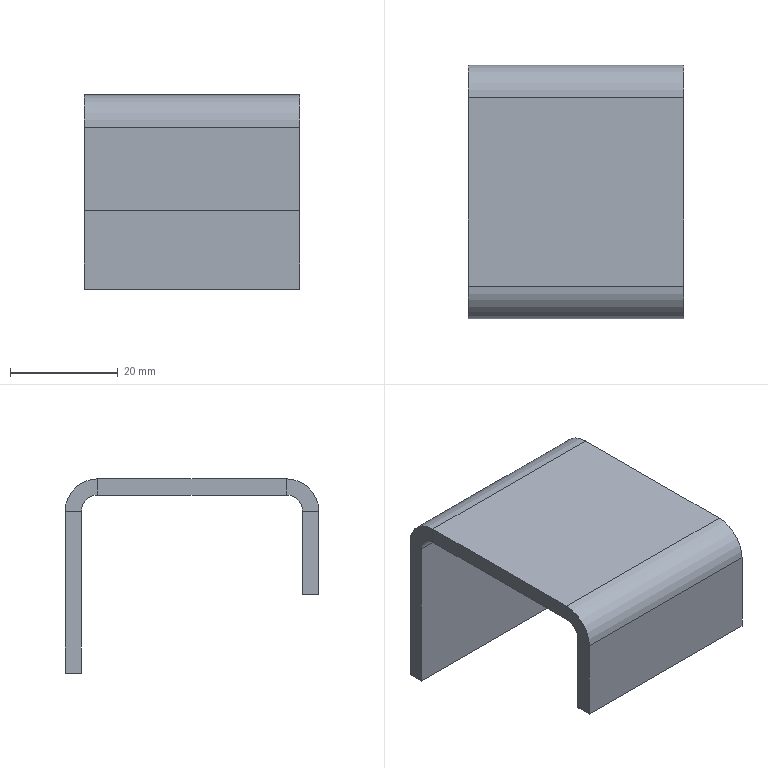Part | SolidWorks | features FlatPattern 1, SMBaseFlange 1, SheetMetal 1 | 1 solid | 22 faces | box 40 x 47 x 36 mm | volume 11356 mm3 | plane 18 | cylinder 4 | commonest cylinder face diameters 6 x2 12 x2
STEP:
#1=CARTESIAN_POINT('',(40.,0.,30.));
#2=VERTEX_POINT('',#1);
#3=CARTESIAN_POINT('',(40.,-3.,30.));
#4=VERTEX_POINT('',#3);
#5=CARTESIAN_POINT('',(40.,0.,30.));
#6=DIRECTION('',(0.,-1.,0.));
#7=VECTOR('',#6,1000.);
#8=LINE('',#5,#7);
#9=EDGE_CURVE('',#2,#4,#8,.T.);
#10=ORIENTED_EDGE('',*,*,#9,.F.);
#11=CARTESIAN_POINT('',(40.,-6.,36.));
#12=VERTEX_POINT('',#11);
#13=CARTESIAN_POINT('',(40.,-6.,30.));
#14=DIRECTION('',(1.,0.,0.));
#15=DIRECTION('',(0.,0.,1.));
#16=AXIS2_PLACEMENT_3D('',#13,#14,#15);
#17=CIRCLE('',#16,6.);
#18=EDGE_CURVE('',#2,#12,#17,.T.);
#19=ORIENTED_EDGE('',*,*,#18,.T.);
#20=CARTESIAN_POINT('',(40.,-6.,33.));
#21=VERTEX_POINT('',#20);
#22=CARTESIAN_POINT('',(40.,-6.,33.));
#23=DIRECTION('',(0.,0.,1.));
#24=VECTOR('',#23,1000.);
#25=LINE('',#22,#24);
#26=EDGE_CURVE('',#21,#12,#25,.T.);
#27=ORIENTED_EDGE('',*,*,#26,.F.);
#28=CARTESIAN_POINT('',(40.,-6.,30.));
#29=DIRECTION('',(1.,0.,0.));
#30=DIRECTION('',(0.,0.,-1.));
#31=AXIS2_PLACEMENT_3D('',#28,#29,#30);
#32=CIRCLE('',#31,3.);
#33=EDGE_CURVE('',#4,#21,#32,.T.);
#34=ORIENTED_EDGE('',*,*,#33,.F.);
#35=EDGE_LOOP('',(#10,#19,#27,#34));
#36=FACE_OUTER_BOUND('',#35,.T.);
#37=CARTESIAN_POINT('',(40.,0.,30.));
#38=DIRECTION('',(1.,0.,0.));
#39=DIRECTION('',(0.,0.,-1.));
#40=AXIS2_PLACEMENT_3D('',#37,#38,#39);
#41=PLANE('',#40);
#42=ADVANCED_FACE('',(#36),#41,.T.);
#43=CARTESIAN_POINT('',(40.,0.,0.));
#44=VERTEX_POINT('',#43);
#45=CARTESIAN_POINT('',(40.,0.,0.));
#46=DIRECTION('',(0.,0.,1.));
#47=VECTOR('',#46,1000.);
#48=LINE('',#45,#47);
#49=EDGE_CURVE('',#44,#2,#48,.T.);
#50=ORIENTED_EDGE('',*,*,#49,.T.);
#51=ORIENTED_EDGE('',*,*,#9,.T.);
#52=CARTESIAN_POINT('',(40.,-3.,0.));
#53=VERTEX_POINT('',#52);
#54=CARTESIAN_POINT('',(40.,-3.,0.));
#55=DIRECTION('',(0.,0.,1.));
#56=VECTOR('',#55,1000.);
#57=LINE('',#54,#56);
#58=EDGE_CURVE('',#53,#4,#57,.T.);
#59=ORIENTED_EDGE('',*,*,#58,.F.);
#60=CARTESIAN_POINT('',(40.,0.,0.));
#61=DIRECTION('',(0.,-1.,0.));
#62=VECTOR('',#61,1000.);
#63=LINE('',#60,#62);
#64=EDGE_CURVE('',#44,#53,#63,.T.);
#65=ORIENTED_EDGE('',*,*,#64,.F.);
#66=EDGE_LOOP('',(#50,#51,#59,#65));
#67=FACE_OUTER_BOUND('',#66,.T.);
#68=CARTESIAN_POINT('',(40.,-6.,33.));
#69=DIRECTION('',(1.,0.,0.));
#70=DIRECTION('',(0.,0.,-1.));
#71=AXIS2_PLACEMENT_3D('',#68,#69,#70);
#72=PLANE('',#71);
#73=ADVANCED_FACE('',(#67),#72,.T.);
#74=CARTESIAN_POINT('',(0.,-6.,36.));
#75=VERTEX_POINT('',#74);
#76=CARTESIAN_POINT('',(0.,-6.,33.));
#77=VERTEX_POINT('',#76);
#78=CARTESIAN_POINT('',(0.,-6.,36.));
#79=DIRECTION('',(0.,0.,-1.));
#80=VECTOR('',#79,1000.);
#81=LINE('',#78,#80);
#82=EDGE_CURVE('',#75,#77,#81,.T.);
#83=ORIENTED_EDGE('',*,*,#82,.F.);
#84=CARTESIAN_POINT('',(0.,0.,30.));
#85=VERTEX_POINT('',#84);
#86=CARTESIAN_POINT('',(0.,-6.,30.));
#87=DIRECTION('',(1.,0.,0.));
#88=DIRECTION('',(0.,0.,1.));
#89=AXIS2_PLACEMENT_3D('',#86,#87,#88);
#90=CIRCLE('',#89,6.);
#91=EDGE_CURVE('',#85,#75,#90,.T.);
#92=ORIENTED_EDGE('',*,*,#91,.F.);
#93=CARTESIAN_POINT('',(0.,-3.,30.));
#94=VERTEX_POINT('',#93);
#95=CARTESIAN_POINT('',(0.,-3.,30.));
#96=DIRECTION('',(0.,1.,0.));
#97=VECTOR('',#96,1000.);
#98=LINE('',#95,#97);
#99=EDGE_CURVE('',#94,#85,#98,.T.);
#100=ORIENTED_EDGE('',*,*,#99,.F.);
#101=CARTESIAN_POINT('',(0.,-6.,30.));
#102=DIRECTION('',(1.,0.,0.));
#103=DIRECTION('',(0.,0.,-1.));
#104=AXIS2_PLACEMENT_3D('',#101,#102,#103);
#105=CIRCLE('',#104,3.);
#106=EDGE_CURVE('',#94,#77,#105,.T.);
#107=ORIENTED_EDGE('',*,*,#106,.T.);
#108=EDGE_LOOP('',(#83,#92,#100,#107));
#109=FACE_OUTER_BOUND('',#108,.T.);
#110=CARTESIAN_POINT('',(0.,-6.,36.));
#111=DIRECTION('',(-1.,0.,0.));
#112=DIRECTION('',(0.,0.,1.));
#113=AXIS2_PLACEMENT_3D('',#110,#111,#112);
#114=PLANE('',#113);
#115=ADVANCED_FACE('',(#109),#114,.T.);
#116=CARTESIAN_POINT('',(0.,-41.,36.));
#117=VERTEX_POINT('',#116);
#118=CARTESIAN_POINT('',(0.,0.,36.));
#119=DIRECTION('',(0.,-1.,0.));
#120=VECTOR('',#119,1000.);
#121=LINE('',#118,#120);
#122=EDGE_CURVE('',#75,#117,#121,.T.);
#123=ORIENTED_EDGE('',*,*,#122,.F.);
#124=ORIENTED_EDGE('',*,*,#82,.T.);
#125=CARTESIAN_POINT('',(0.,-41.,33.));
#126=VERTEX_POINT('',#125);
#127=CARTESIAN_POINT('',(0.,0.,33.));
#128=DIRECTION('',(0.,-1.,0.));
#129=VECTOR('',#128,1000.);
#130=LINE('',#127,#129);
#131=EDGE_CURVE('',#77,#126,#130,.T.);
#132=ORIENTED_EDGE('',*,*,#131,.T.);
#133=CARTESIAN_POINT('',(0.,-41.,33.));
#134=DIRECTION('',(0.,0.,1.));
#135=VECTOR('',#134,1000.);
#136=LINE('',#133,#135);
#137=EDGE_CURVE('',#126,#117,#136,.T.);
#138=ORIENTED_EDGE('',*,*,#137,.T.);
#139=EDGE_LOOP('',(#123,#124,#132,#138));
#140=FACE_OUTER_BOUND('',#139,.T.);
#141=CARTESIAN_POINT('',(0.,-3.,30.));
#142=DIRECTION('',(-1.,0.,0.));
#143=DIRECTION('',(0.,0.,1.));
#144=AXIS2_PLACEMENT_3D('',#141,#142,#143);
#145=PLANE('',#144);
#146=ADVANCED_FACE('',(#140),#145,.T.);
#147=CARTESIAN_POINT('',(40.,-41.,36.));
#148=VERTEX_POINT('',#147);
#149=CARTESIAN_POINT('',(40.,-41.,33.));
#150=VERTEX_POINT('',#149);
#151=CARTESIAN_POINT('',(40.,-41.,36.));
#152=DIRECTION('',(0.,0.,-1.));
#153=VECTOR('',#152,1000.);
#154=LINE('',#151,#153);
#155=EDGE_CURVE('',#148,#150,#154,.T.);
#156=ORIENTED_EDGE('',*,*,#155,.F.);
#157=CARTESIAN_POINT('',(40.,-47.,30.));
#158=VERTEX_POINT('',#157);
#159=CARTESIAN_POINT('',(40.,-41.,30.));
#160=DIRECTION('',(1.,0.,0.));
#161=DIRECTION('',(0.,0.,1.));
#162=AXIS2_PLACEMENT_3D('',#159,#160,#161);
#163=CIRCLE('',#162,6.);
#164=EDGE_CURVE('',#148,#158,#163,.T.);
#165=ORIENTED_EDGE('',*,*,#164,.T.);
#166=CARTESIAN_POINT('',(40.,-44.,30.));
#167=VERTEX_POINT('',#166);
#168=CARTESIAN_POINT('',(40.,-44.,30.));
#169=DIRECTION('',(0.,-1.,0.));
#170=VECTOR('',#169,1000.);
#171=LINE('',#168,#170);
#172=EDGE_CURVE('',#167,#158,#171,.T.);
#173=ORIENTED_EDGE('',*,*,#172,.F.);
#174=CARTESIAN_POINT('',(40.,-41.,30.));
#175=DIRECTION('',(1.,0.,0.));
#176=DIRECTION('',(0.,0.,-1.));
#177=AXIS2_PLACEMENT_3D('',#174,#175,#176);
#178=CIRCLE('',#177,3.);
#179=EDGE_CURVE('',#150,#167,#178,.T.);
#180=ORIENTED_EDGE('',*,*,#179,.F.);
#181=EDGE_LOOP('',(#156,#165,#173,#180));
#182=FACE_OUTER_BOUND('',#181,.T.);
#183=CARTESIAN_POINT('',(40.,-41.,36.));
#184=DIRECTION('',(1.,0.,0.));
#185=DIRECTION('',(0.,0.,-1.));
#186=AXIS2_PLACEMENT_3D('',#183,#184,#185);
#187=PLANE('',#186);
#188=ADVANCED_FACE('',(#182),#187,.T.);
#189=CARTESIAN_POINT('',(40.,0.,36.));
#190=DIRECTION('',(0.,-1.,0.));
#191=VECTOR('',#190,1000.);
#192=LINE('',#189,#191);
#193=EDGE_CURVE('',#12,#148,#192,.T.);
#194=ORIENTED_EDGE('',*,*,#193,.T.);
#195=ORIENTED_EDGE('',*,*,#155,.T.);
#196=CARTESIAN_POINT('',(40.,0.,33.));
#197=DIRECTION('',(0.,-1.,0.));
#198=VECTOR('',#197,1000.);
#199=LINE('',#196,#198);
#200=EDGE_CURVE('',#21,#150,#199,.T.);
#201=ORIENTED_EDGE('',*,*,#200,.F.);
#202=ORIENTED_EDGE('',*,*,#26,.T.);
#203=EDGE_LOOP('',(#194,#195,#201,#202));
#204=FACE_OUTER_BOUND('',#203,.T.);
#205=CARTESIAN_POINT('',(40.,-44.,30.));
#206=DIRECTION('',(1.,0.,0.));
#207=DIRECTION('',(0.,0.,-1.));
#208=AXIS2_PLACEMENT_3D('',#205,#206,#207);
#209=PLANE('',#208);
#210=ADVANCED_FACE('',(#204),#209,.T.);
#211=CARTESIAN_POINT('',(0.,-47.,30.));
#212=VERTEX_POINT('',#211);
#213=CARTESIAN_POINT('',(0.,-44.,30.));
#214=VERTEX_POINT('',#213);
#215=CARTESIAN_POINT('',(0.,-47.,30.));
#216=DIRECTION('',(0.,1.,0.));
#217=VECTOR('',#216,1000.);
#218=LINE('',#215,#217);
#219=EDGE_CURVE('',#212,#214,#218,.T.);
#220=ORIENTED_EDGE('',*,*,#219,.F.);
#221=CARTESIAN_POINT('',(0.,-41.,30.));
#222=DIRECTION('',(1.,0.,0.));
#223=DIRECTION('',(0.,0.,1.));
#224=AXIS2_PLACEMENT_3D('',#221,#222,#223);
#225=CIRCLE('',#224,6.);
#226=EDGE_CURVE('',#117,#212,#225,.T.);
#227=ORIENTED_EDGE('',*,*,#226,.F.);
#228=ORIENTED_EDGE('',*,*,#137,.F.);
#229=CARTESIAN_POINT('',(0.,-41.,30.));
#230=DIRECTION('',(1.,0.,0.));
#231=DIRECTION('',(0.,0.,-1.));
#232=AXIS2_PLACEMENT_3D('',#229,#230,#231);
#233=CIRCLE('',#232,3.);
#234=EDGE_CURVE('',#126,#214,#233,.T.);
#235=ORIENTED_EDGE('',*,*,#234,.T.);
#236=EDGE_LOOP('',(#220,#227,#228,#235));
#237=FACE_OUTER_BOUND('',#236,.T.);
#238=CARTESIAN_POINT('',(0.,-47.,30.));
#239=DIRECTION('',(-1.,0.,0.));
#240=DIRECTION('',(0.,0.,1.));
#241=AXIS2_PLACEMENT_3D('',#238,#239,#240);
#242=PLANE('',#241);
#243=ADVANCED_FACE('',(#237),#242,.T.);
#244=CARTESIAN_POINT('',(0.,-47.,14.5));
#245=VERTEX_POINT('',#244);
#246=CARTESIAN_POINT('',(0.,-47.,36.));
#247=DIRECTION('',(0.,0.,-1.));
#248=VECTOR('',#247,1000.);
#249=LINE('',#246,#248);
#250=EDGE_CURVE('',#212,#245,#249,.T.);
#251=ORIENTED_EDGE('',*,*,#250,.F.);
#252=ORIENTED_EDGE('',*,*,#219,.T.);
#253=CARTESIAN_POINT('',(0.,-44.,14.5));
#254=VERTEX_POINT('',#253);
#255=CARTESIAN_POINT('',(0.,-44.,36.));
#256=DIRECTION('',(0.,0.,-1.));
#257=VECTOR('',#256,1000.);
#258=LINE('',#255,#257);
#259=EDGE_CURVE('',#214,#254,#258,.T.);
#260=ORIENTED_EDGE('',*,*,#259,.T.);
#261=CARTESIAN_POINT('',(0.,-44.,14.5));
#262=DIRECTION('',(0.,-1.,0.));
#263=VECTOR('',#262,1000.);
#264=LINE('',#261,#263);
#265=EDGE_CURVE('',#254,#245,#264,.T.);
#266=ORIENTED_EDGE('',*,*,#265,.T.);
#267=EDGE_LOOP('',(#251,#252,#260,#266));
#268=FACE_OUTER_BOUND('',#267,.T.);
#269=CARTESIAN_POINT('',(0.,-41.,33.));
#270=DIRECTION('',(-1.,0.,0.));
#271=DIRECTION('',(0.,0.,1.));
#272=AXIS2_PLACEMENT_3D('',#269,#270,#271);
#273=PLANE('',#272);
#274=ADVANCED_FACE('',(#268),#273,.T.);
#275=ORIENTED_EDGE('',*,*,#250,.T.);
#276=CARTESIAN_POINT('',(40.,-47.,14.5));
#277=VERTEX_POINT('',#276);
#278=CARTESIAN_POINT('',(40.,-47.,14.5));
#279=DIRECTION('',(-1.,0.,0.));
#280=VECTOR('',#279,1000.);
#281=LINE('',#278,#280);
#282=EDGE_CURVE('',#277,#245,#281,.T.);
#283=ORIENTED_EDGE('',*,*,#282,.F.);
#284=CARTESIAN_POINT('',(40.,-47.,36.));
#285=DIRECTION('',(0.,0.,-1.));
#286=VECTOR('',#285,1000.);
#287=LINE('',#284,#286);
#288=EDGE_CURVE('',#158,#277,#287,.T.);
#289=ORIENTED_EDGE('',*,*,#288,.F.);
#290=CARTESIAN_POINT('',(40.,-47.,30.));
#291=DIRECTION('',(-1.,0.,0.));
#292=VECTOR('',#291,1000.);
#293=LINE('',#290,#292);
#294=EDGE_CURVE('',#158,#212,#293,.T.);
#295=ORIENTED_EDGE('',*,*,#294,.T.);
#296=EDGE_LOOP('',(#275,#283,#289,#295));
#297=FACE_OUTER_BOUND('',#296,.T.);
#298=CARTESIAN_POINT('',(40.,-47.,36.));
#299=DIRECTION('',(0.,1.,0.));
#300=DIRECTION('',(0.,0.,1.));
#301=AXIS2_PLACEMENT_3D('',#298,#299,#300);
#302=PLANE('',#301);
#303=ADVANCED_FACE('',(#297),#302,.F.);
#304=ORIENTED_EDGE('',*,*,#265,.F.);
#305=CARTESIAN_POINT('',(40.,-44.,14.5));
#306=VERTEX_POINT('',#305);
#307=CARTESIAN_POINT('',(40.,-44.,14.5));
#308=DIRECTION('',(-1.,0.,0.));
#309=VECTOR('',#308,1000.);
#310=LINE('',#307,#309);
#311=EDGE_CURVE('',#306,#254,#310,.T.);
#312=ORIENTED_EDGE('',*,*,#311,.F.);
#313=CARTESIAN_POINT('',(40.,-44.,14.5));
#314=DIRECTION('',(0.,-1.,0.));
#315=VECTOR('',#314,1000.);
#316=LINE('',#313,#315);
#317=EDGE_CURVE('',#306,#277,#316,.T.);
#318=ORIENTED_EDGE('',*,*,#317,.T.);
#319=ORIENTED_EDGE('',*,*,#282,.T.);
#320=EDGE_LOOP('',(#304,#312,#318,#319));
#321=FACE_OUTER_BOUND('',#320,.T.);
#322=CARTESIAN_POINT('',(40.,-44.,14.5));
#323=DIRECTION('',(0.,0.,-1.));
#324=DIRECTION('',(0.,1.,0.));
#325=AXIS2_PLACEMENT_3D('',#322,#323,#324);
#326=PLANE('',#325);
#327=ADVANCED_FACE('',(#321),#326,.T.);
#328=ORIENTED_EDGE('',*,*,#259,.F.);
#329=CARTESIAN_POINT('',(40.,-44.,30.));
#330=DIRECTION('',(-1.,0.,0.));
#331=VECTOR('',#330,1000.);
#332=LINE('',#329,#331);
#333=EDGE_CURVE('',#167,#214,#332,.T.);
#334=ORIENTED_EDGE('',*,*,#333,.F.);
#335=CARTESIAN_POINT('',(40.,-44.,36.));
#336=DIRECTION('',(0.,0.,-1.));
#337=VECTOR('',#336,1000.);
#338=LINE('',#335,#337);
#339=EDGE_CURVE('',#167,#306,#338,.T.);
#340=ORIENTED_EDGE('',*,*,#339,.T.);
#341=ORIENTED_EDGE('',*,*,#311,.T.);
#342=EDGE_LOOP('',(#328,#334,#340,#341));
#343=FACE_OUTER_BOUND('',#342,.T.);
#344=CARTESIAN_POINT('',(40.,-44.,36.));
#345=DIRECTION('',(0.,1.,0.));
#346=DIRECTION('',(0.,0.,1.));
#347=AXIS2_PLACEMENT_3D('',#344,#345,#346);
#348=PLANE('',#347);
#349=ADVANCED_FACE('',(#343),#348,.T.);
#350=ORIENTED_EDGE('',*,*,#234,.F.);
#351=CARTESIAN_POINT('',(40.,-41.,33.));
#352=DIRECTION('',(-1.,0.,0.));
#353=VECTOR('',#352,1000.);
#354=LINE('',#351,#353);
#355=EDGE_CURVE('',#150,#126,#354,.T.);
#356=ORIENTED_EDGE('',*,*,#355,.F.);
#357=ORIENTED_EDGE('',*,*,#179,.T.);
#358=ORIENTED_EDGE('',*,*,#333,.T.);
#359=EDGE_LOOP('',(#350,#356,#357,#358));
#360=FACE_OUTER_BOUND('',#359,.T.);
#361=CARTESIAN_POINT('',(40.,-41.,30.));
#362=DIRECTION('',(-1.,0.,0.));
#363=DIRECTION('',(0.,0.,1.));
#364=AXIS2_PLACEMENT_3D('',#361,#362,#363);
#365=CYLINDRICAL_SURFACE('',#364,3.);
#366=ADVANCED_FACE('',(#360),#365,.F.);
#367=ORIENTED_EDGE('',*,*,#131,.F.);
#368=CARTESIAN_POINT('',(40.,-6.,33.));
#369=DIRECTION('',(-1.,0.,0.));
#370=VECTOR('',#369,1000.);
#371=LINE('',#368,#370);
#372=EDGE_CURVE('',#21,#77,#371,.T.);
#373=ORIENTED_EDGE('',*,*,#372,.F.);
#374=ORIENTED_EDGE('',*,*,#200,.T.);
#375=ORIENTED_EDGE('',*,*,#355,.T.);
#376=EDGE_LOOP('',(#367,#373,#374,#375));
#377=FACE_OUTER_BOUND('',#376,.T.);
#378=CARTESIAN_POINT('',(40.,0.,33.));
#379=DIRECTION('',(0.,0.,-1.));
#380=DIRECTION('',(-1.,0.,0.));
#381=AXIS2_PLACEMENT_3D('',#378,#379,#380);
#382=PLANE('',#381);
#383=ADVANCED_FACE('',(#377),#382,.T.);
#384=ORIENTED_EDGE('',*,*,#106,.F.);
#385=CARTESIAN_POINT('',(40.,-3.,30.));
#386=DIRECTION('',(-1.,0.,0.));
#387=VECTOR('',#386,1000.);
#388=LINE('',#385,#387);
#389=EDGE_CURVE('',#4,#94,#388,.T.);
#390=ORIENTED_EDGE('',*,*,#389,.F.);
#391=ORIENTED_EDGE('',*,*,#33,.T.);
#392=ORIENTED_EDGE('',*,*,#372,.T.);
#393=EDGE_LOOP('',(#384,#390,#391,#392));
#394=FACE_OUTER_BOUND('',#393,.T.);
#395=CARTESIAN_POINT('',(40.,-6.,30.));
#396=DIRECTION('',(-1.,0.,0.));
#397=DIRECTION('',(0.,0.,1.));
#398=AXIS2_PLACEMENT_3D('',#395,#396,#397);
#399=CYLINDRICAL_SURFACE('',#398,3.);
#400=ADVANCED_FACE('',(#394),#399,.F.);
#401=CARTESIAN_POINT('',(0.,-3.,0.));
#402=VERTEX_POINT('',#401);
#403=CARTESIAN_POINT('',(0.,-3.,0.));
#404=DIRECTION('',(0.,0.,1.));
#405=VECTOR('',#404,1000.);
#406=LINE('',#403,#405);
#407=EDGE_CURVE('',#402,#94,#406,.T.);
#408=ORIENTED_EDGE('',*,*,#407,.F.);
#409=CARTESIAN_POINT('',(40.,-3.,0.));
#410=DIRECTION('',(-1.,0.,0.));
#411=VECTOR('',#410,1000.);
#412=LINE('',#409,#411);
#413=EDGE_CURVE('',#53,#402,#412,.T.);
#414=ORIENTED_EDGE('',*,*,#413,.F.);
#415=ORIENTED_EDGE('',*,*,#58,.T.);
#416=ORIENTED_EDGE('',*,*,#389,.T.);
#417=EDGE_LOOP('',(#408,#414,#415,#416));
#418=FACE_OUTER_BOUND('',#417,.T.);
#419=CARTESIAN_POINT('',(40.,-3.,0.));
#420=DIRECTION('',(0.,-1.,0.));
#421=DIRECTION('',(0.,0.,-1.));
#422=AXIS2_PLACEMENT_3D('',#419,#420,#421);
#423=PLANE('',#422);
#424=ADVANCED_FACE('',(#418),#423,.T.);
#425=CARTESIAN_POINT('',(0.,0.,0.));
#426=VERTEX_POINT('',#425);
#427=CARTESIAN_POINT('',(0.,0.,0.));
#428=DIRECTION('',(0.,-1.,0.));
#429=VECTOR('',#428,1000.);
#430=LINE('',#427,#429);
#431=EDGE_CURVE('',#426,#402,#430,.T.);
#432=ORIENTED_EDGE('',*,*,#431,.F.);
#433=CARTESIAN_POINT('',(40.,0.,0.));
#434=DIRECTION('',(-1.,0.,0.));
#435=VECTOR('',#434,1000.);
#436=LINE('',#433,#435);
#437=EDGE_CURVE('',#44,#426,#436,.T.);
#438=ORIENTED_EDGE('',*,*,#437,.F.);
#439=ORIENTED_EDGE('',*,*,#64,.T.);
#440=ORIENTED_EDGE('',*,*,#413,.T.);
#441=EDGE_LOOP('',(#432,#438,#439,#440));
#442=FACE_OUTER_BOUND('',#441,.T.);
#443=CARTESIAN_POINT('',(40.,0.,0.));
#444=DIRECTION('',(0.,0.,-1.));
#445=DIRECTION('',(-1.,0.,0.));
#446=AXIS2_PLACEMENT_3D('',#443,#444,#445);
#447=PLANE('',#446);
#448=ADVANCED_FACE('',(#442),#447,.T.);
#449=CARTESIAN_POINT('',(0.,0.,0.));
#450=DIRECTION('',(0.,0.,1.));
#451=VECTOR('',#450,1000.);
#452=LINE('',#449,#451);
#453=EDGE_CURVE('',#426,#85,#452,.T.);
#454=ORIENTED_EDGE('',*,*,#453,.T.);
#455=CARTESIAN_POINT('',(40.,0.,30.));
#456=DIRECTION('',(-1.,0.,0.));
#457=VECTOR('',#456,1000.);
#458=LINE('',#455,#457);
#459=EDGE_CURVE('',#2,#85,#458,.T.);
#460=ORIENTED_EDGE('',*,*,#459,.F.);
#461=ORIENTED_EDGE('',*,*,#49,.F.);
#462=ORIENTED_EDGE('',*,*,#437,.T.);
#463=EDGE_LOOP('',(#454,#460,#461,#462));
#464=FACE_OUTER_BOUND('',#463,.T.);
#465=CARTESIAN_POINT('',(40.,0.,0.));
#466=DIRECTION('',(0.,-1.,0.));
#467=DIRECTION('',(0.,0.,-1.));
#468=AXIS2_PLACEMENT_3D('',#465,#466,#467);
#469=PLANE('',#468);
#470=ADVANCED_FACE('',(#464),#469,.F.);
#471=ORIENTED_EDGE('',*,*,#91,.T.);
#472=CARTESIAN_POINT('',(40.,-6.,36.));
#473=DIRECTION('',(-1.,0.,0.));
#474=VECTOR('',#473,1000.);
#475=LINE('',#472,#474);
#476=EDGE_CURVE('',#12,#75,#475,.T.);
#477=ORIENTED_EDGE('',*,*,#476,.F.);
#478=ORIENTED_EDGE('',*,*,#18,.F.);
#479=ORIENTED_EDGE('',*,*,#459,.T.);
#480=EDGE_LOOP('',(#471,#477,#478,#479));
#481=FACE_OUTER_BOUND('',#480,.T.);
#482=CARTESIAN_POINT('',(40.,-6.,30.));
#483=DIRECTION('',(-1.,0.,0.));
#484=DIRECTION('',(0.,0.,1.));
#485=AXIS2_PLACEMENT_3D('',#482,#483,#484);
#486=CYLINDRICAL_SURFACE('',#485,6.);
#487=ADVANCED_FACE('',(#481),#486,.T.);
#488=ORIENTED_EDGE('',*,*,#122,.T.);
#489=CARTESIAN_POINT('',(40.,-41.,36.));
#490=DIRECTION('',(-1.,0.,0.));
#491=VECTOR('',#490,1000.);
#492=LINE('',#489,#491);
#493=EDGE_CURVE('',#148,#117,#492,.T.);
#494=ORIENTED_EDGE('',*,*,#493,.F.);
#495=ORIENTED_EDGE('',*,*,#193,.F.);
#496=ORIENTED_EDGE('',*,*,#476,.T.);
#497=EDGE_LOOP('',(#488,#494,#495,#496));
#498=FACE_OUTER_BOUND('',#497,.T.);
#499=CARTESIAN_POINT('',(40.,0.,36.));
#500=DIRECTION('',(0.,0.,-1.));
#501=DIRECTION('',(-1.,0.,0.));
#502=AXIS2_PLACEMENT_3D('',#499,#500,#501);
#503=PLANE('',#502);
#504=ADVANCED_FACE('',(#498),#503,.F.);
#505=ORIENTED_EDGE('',*,*,#226,.T.);
#506=ORIENTED_EDGE('',*,*,#294,.F.);
#507=ORIENTED_EDGE('',*,*,#164,.F.);
#508=ORIENTED_EDGE('',*,*,#493,.T.);
#509=EDGE_LOOP('',(#505,#506,#507,#508));
#510=FACE_OUTER_BOUND('',#509,.T.);
#511=CARTESIAN_POINT('',(40.,-41.,30.));
#512=DIRECTION('',(-1.,0.,0.));
#513=DIRECTION('',(0.,0.,1.));
#514=AXIS2_PLACEMENT_3D('',#511,#512,#513);
#515=CYLINDRICAL_SURFACE('',#514,6.);
#516=ADVANCED_FACE('',(#510),#515,.T.);
#517=ORIENTED_EDGE('',*,*,#288,.T.);
#518=ORIENTED_EDGE('',*,*,#317,.F.);
#519=ORIENTED_EDGE('',*,*,#339,.F.);
#520=ORIENTED_EDGE('',*,*,#172,.T.);
#521=EDGE_LOOP('',(#517,#518,#519,#520));
#522=FACE_OUTER_BOUND('',#521,.T.);
#523=CARTESIAN_POINT('',(40.,-41.,30.));
#524=DIRECTION('',(1.,0.,0.));
#525=DIRECTION('',(0.,0.,-1.));
#526=AXIS2_PLACEMENT_3D('',#523,#524,#525);
#527=PLANE('',#526);
#528=ADVANCED_FACE('',(#522),#527,.T.);
#529=ORIENTED_EDGE('',*,*,#407,.T.);
#530=ORIENTED_EDGE('',*,*,#99,.T.);
#531=ORIENTED_EDGE('',*,*,#453,.F.);
#532=ORIENTED_EDGE('',*,*,#431,.T.);
#533=EDGE_LOOP('',(#529,#530,#531,#532));
#534=FACE_OUTER_BOUND('',#533,.T.);
#535=CARTESIAN_POINT('',(0.,-41.,30.));
#536=DIRECTION('',(1.,0.,0.));
#537=DIRECTION('',(0.,0.,-1.));
#538=AXIS2_PLACEMENT_3D('',#535,#536,#537);
#539=PLANE('',#538);
#540=ADVANCED_FACE('',(#534),#539,.F.);
#541=CLOSED_SHELL('',(#42,#73,#115,#146,#188,#210,#243,#274,#303,#327,#349,#366,#383,#400,#424,#448,#470,#487,#504,#516,#528,#540));
#542=MANIFOLD_SOLID_BREP('',#541);
#543=CARTESIAN_POINT('',(0.,0.,0.));
#544=DIRECTION('',(0.,0.,1.));
#545=DIRECTION('',(1.,0.,0.));
#546=AXIS2_PLACEMENT_3D('',#543,#544,#545);
#547=(LENGTH_UNIT()NAMED_UNIT(*)SI_UNIT(.MILLI.,.METRE.));
#548=UNCERTAINTY_MEASURE_WITH_UNIT(LENGTH_MEASURE(0.00001),#547,'','');
#549=(NAMED_UNIT(*)PLANE_ANGLE_UNIT()SI_UNIT($,.RADIAN.));
#550=(NAMED_UNIT(*)SI_UNIT($,.STERADIAN.)SOLID_ANGLE_UNIT());
#551=(GEOMETRIC_REPRESENTATION_CONTEXT(3)GLOBAL_UNCERTAINTY_ASSIGNED_CONTEXT((#548))GLOBAL_UNIT_ASSIGNED_CONTEXT((#547,#549,#550))REPRESENTATION_CONTEXT('',''));
#552=ADVANCED_BREP_SHAPE_REPRESENTATION('',(#542,#546),#551);